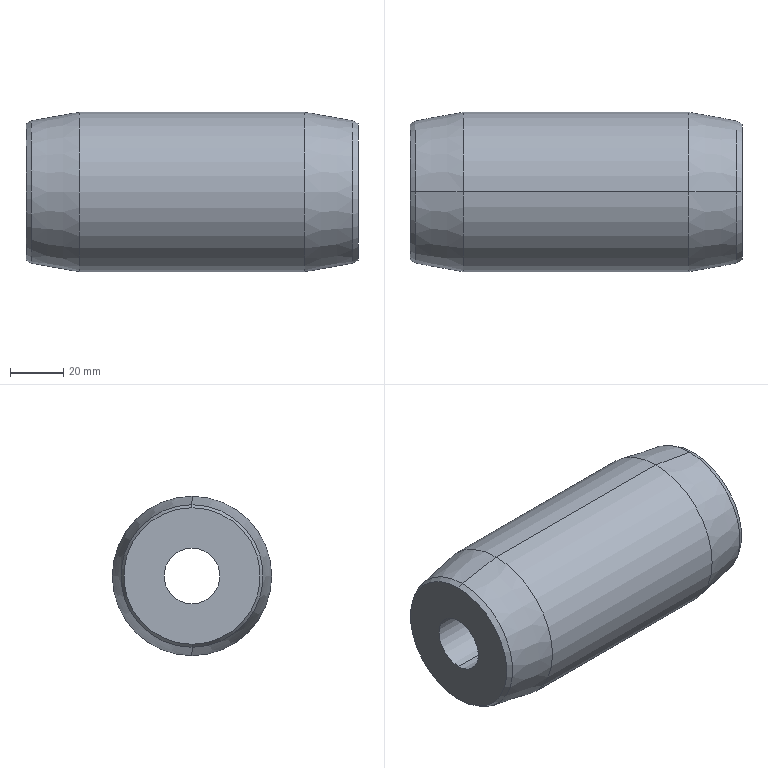Part | SolidWorks | features 3DProfileFeature 1, Chamfer 1, HoleWzd 1, ICE 1, Revolution 1 | 1 solid | 14 faces | box 125 x 60 x 60 mm | volume 297103 mm3 | cone 8 | cylinder 4 | plane 2 | commonest cylinder face diameters 21 x2 60 x2
STEP:
#1=CARTESIAN_POINT('',(125.,0.,-25.684));
#2=VERTEX_POINT('',#1);
#3=CARTESIAN_POINT('',(125.,0.,25.684));
#4=VERTEX_POINT('',#3);
#5=CARTESIAN_POINT('',(125.,0.,0.));
#6=DIRECTION('',(1.,0.,0.));
#7=DIRECTION('',(0.,0.,1.));
#8=AXIS2_PLACEMENT_3D('',#5,#6,#7);
#9=CIRCLE('',#8,25.684);
#10=EDGE_CURVE('',#2,#4,#9,.T.);
#11=ORIENTED_EDGE('',*,*,#10,.F.);
#12=CARTESIAN_POINT('',(123.03,0.,-26.821));
#13=VERTEX_POINT('',#12);
#14=CARTESIAN_POINT('',(123.03,0.,-26.821));
#15=DIRECTION('',(-0.866,0.,-0.5));
#16=VECTOR('',#15,1000.);
#17=LINE('',#14,#16);
#18=EDGE_CURVE('',#2,#13,#17,.T.);
#19=ORIENTED_EDGE('',*,*,#18,.T.);
#20=CARTESIAN_POINT('',(123.03,0.,26.821));
#21=VERTEX_POINT('',#20);
#22=CARTESIAN_POINT('',(123.03,0.,0.));
#23=DIRECTION('',(-1.,0.,0.));
#24=DIRECTION('',(0.,0.,-1.));
#25=AXIS2_PLACEMENT_3D('',#22,#23,#24);
#26=CIRCLE('',#25,26.821);
#27=EDGE_CURVE('',#21,#13,#26,.T.);
#28=ORIENTED_EDGE('',*,*,#27,.F.);
#29=CARTESIAN_POINT('',(123.03,0.,26.821));
#30=DIRECTION('',(-0.866,0.,0.5));
#31=VECTOR('',#30,1000.);
#32=LINE('',#29,#31);
#33=EDGE_CURVE('',#4,#21,#32,.T.);
#34=ORIENTED_EDGE('',*,*,#33,.F.);
#35=EDGE_LOOP('',(#11,#19,#28,#34));
#36=FACE_OUTER_BOUND('',#35,.T.);
#37=CARTESIAN_POINT('',(123.03,0.,0.));
#38=DIRECTION('',(-1.,0.,0.));
#39=DIRECTION('',(0.,0.,1.));
#40=AXIS2_PLACEMENT_3D('',#37,#38,#39);
#41=CONICAL_SURFACE('',#40,26.821,0.5236);
#42=ADVANCED_FACE('',(#36),#41,.T.);
#43=CARTESIAN_POINT('',(0.,0.,25.684));
#44=VERTEX_POINT('',#43);
#45=CARTESIAN_POINT('',(0.,0.,-25.684));
#46=VERTEX_POINT('',#45);
#47=CARTESIAN_POINT('',(0.,0.,0.));
#48=DIRECTION('',(-1.,0.,0.));
#49=DIRECTION('',(0.,0.,-1.));
#50=AXIS2_PLACEMENT_3D('',#47,#48,#49);
#51=CIRCLE('',#50,25.684);
#52=EDGE_CURVE('',#44,#46,#51,.T.);
#53=ORIENTED_EDGE('',*,*,#52,.F.);
#54=CARTESIAN_POINT('',(1.97,0.,26.821));
#55=VERTEX_POINT('',#54);
#56=CARTESIAN_POINT('',(0.,0.,25.684));
#57=DIRECTION('',(0.866,0.,0.5));
#58=VECTOR('',#57,1000.);
#59=LINE('',#56,#58);
#60=EDGE_CURVE('',#44,#55,#59,.T.);
#61=ORIENTED_EDGE('',*,*,#60,.T.);
#62=CARTESIAN_POINT('',(1.97,0.,-26.821));
#63=VERTEX_POINT('',#62);
#64=CARTESIAN_POINT('',(1.97,0.,0.));
#65=DIRECTION('',(1.,0.,0.));
#66=DIRECTION('',(0.,0.,1.));
#67=AXIS2_PLACEMENT_3D('',#64,#65,#66);
#68=CIRCLE('',#67,26.821);
#69=EDGE_CURVE('',#63,#55,#68,.T.);
#70=ORIENTED_EDGE('',*,*,#69,.F.);
#71=CARTESIAN_POINT('',(0.,0.,-25.684));
#72=DIRECTION('',(0.866,0.,-0.5));
#73=VECTOR('',#72,1000.);
#74=LINE('',#71,#73);
#75=EDGE_CURVE('',#46,#63,#74,.T.);
#76=ORIENTED_EDGE('',*,*,#75,.F.);
#77=EDGE_LOOP('',(#53,#61,#70,#76));
#78=FACE_OUTER_BOUND('',#77,.T.);
#79=CARTESIAN_POINT('',(0.,0.,0.));
#80=DIRECTION('',(1.,0.,0.));
#81=DIRECTION('',(0.,0.,-1.));
#82=AXIS2_PLACEMENT_3D('',#79,#80,#81);
#83=CONICAL_SURFACE('',#82,25.684,0.5236);
#84=ADVANCED_FACE('',(#78),#83,.T.);
#85=CARTESIAN_POINT('',(0.,0.,10.5));
#86=VERTEX_POINT('',#85);
#87=CARTESIAN_POINT('',(0.,0.,-10.5));
#88=VERTEX_POINT('',#87);
#89=CARTESIAN_POINT('',(0.,0.,0.));
#90=DIRECTION('',(1.,0.,0.));
#91=DIRECTION('',(0.,0.,-1.));
#92=AXIS2_PLACEMENT_3D('',#89,#90,#91);
#93=CIRCLE('',#92,10.5);
#94=EDGE_CURVE('',#86,#88,#93,.T.);
#95=ORIENTED_EDGE('',*,*,#94,.F.);
#96=CARTESIAN_POINT('',(125.,0.,10.5));
#97=VERTEX_POINT('',#96);
#98=CARTESIAN_POINT('',(0.,0.,10.5));
#99=DIRECTION('',(1.,0.,0.));
#100=VECTOR('',#99,1000.);
#101=LINE('',#98,#100);
#102=EDGE_CURVE('',#86,#97,#101,.T.);
#103=ORIENTED_EDGE('',*,*,#102,.T.);
#104=CARTESIAN_POINT('',(125.,0.,-10.5));
#105=VERTEX_POINT('',#104);
#106=CARTESIAN_POINT('',(125.,0.,0.));
#107=DIRECTION('',(1.,0.,0.));
#108=DIRECTION('',(0.,0.,-1.));
#109=AXIS2_PLACEMENT_3D('',#106,#107,#108);
#110=CIRCLE('',#109,10.5);
#111=EDGE_CURVE('',#97,#105,#110,.T.);
#112=ORIENTED_EDGE('',*,*,#111,.T.);
#113=CARTESIAN_POINT('',(0.,0.,-10.5));
#114=DIRECTION('',(1.,0.,0.));
#115=VECTOR('',#114,1000.);
#116=LINE('',#113,#115);
#117=EDGE_CURVE('',#88,#105,#116,.T.);
#118=ORIENTED_EDGE('',*,*,#117,.F.);
#119=EDGE_LOOP('',(#95,#103,#112,#118));
#120=FACE_OUTER_BOUND('',#119,.T.);
#121=CARTESIAN_POINT('',(0.,0.,0.));
#122=DIRECTION('',(1.,0.,0.));
#123=DIRECTION('',(0.,0.,-1.));
#124=AXIS2_PLACEMENT_3D('',#121,#122,#123);
#125=CYLINDRICAL_SURFACE('',#124,10.5);
#126=ADVANCED_FACE('',(#120),#125,.F.);
#127=ORIENTED_EDGE('',*,*,#69,.T.);
#128=CARTESIAN_POINT('',(20.,0.,30.));
#129=VERTEX_POINT('',#128);
#130=CARTESIAN_POINT('',(20.,0.,30.));
#131=DIRECTION('',(0.9848,0.,0.1736));
#132=VECTOR('',#131,1000.);
#133=LINE('',#130,#132);
#134=EDGE_CURVE('',#55,#129,#133,.T.);
#135=ORIENTED_EDGE('',*,*,#134,.T.);
#136=CARTESIAN_POINT('',(20.,0.,-30.));
#137=VERTEX_POINT('',#136);
#138=CARTESIAN_POINT('',(20.,0.,0.));
#139=DIRECTION('',(-1.,0.,0.));
#140=DIRECTION('',(0.,0.,1.));
#141=AXIS2_PLACEMENT_3D('',#138,#139,#140);
#142=CIRCLE('',#141,30.);
#143=EDGE_CURVE('',#129,#137,#142,.T.);
#144=ORIENTED_EDGE('',*,*,#143,.T.);
#145=CARTESIAN_POINT('',(20.,0.,-30.));
#146=DIRECTION('',(0.9848,0.,-0.1736));
#147=VECTOR('',#146,1000.);
#148=LINE('',#145,#147);
#149=EDGE_CURVE('',#63,#137,#148,.T.);
#150=ORIENTED_EDGE('',*,*,#149,.F.);
#151=EDGE_LOOP('',(#127,#135,#144,#150));
#152=FACE_OUTER_BOUND('',#151,.T.);
#153=CARTESIAN_POINT('',(20.,0.,0.));
#154=DIRECTION('',(1.,0.,0.));
#155=DIRECTION('',(0.,0.,-1.));
#156=AXIS2_PLACEMENT_3D('',#153,#154,#155);
#157=CONICAL_SURFACE('',#156,30.,0.1745);
#158=ADVANCED_FACE('',(#152),#157,.T.);
#159=CARTESIAN_POINT('',(105.,0.,30.));
#160=VERTEX_POINT('',#159);
#161=CARTESIAN_POINT('',(105.,0.,-30.));
#162=VERTEX_POINT('',#161);
#163=CARTESIAN_POINT('',(105.,0.,0.));
#164=DIRECTION('',(-1.,0.,0.));
#165=DIRECTION('',(0.,0.,1.));
#166=AXIS2_PLACEMENT_3D('',#163,#164,#165);
#167=CIRCLE('',#166,30.);
#168=EDGE_CURVE('',#160,#162,#167,.T.);
#169=ORIENTED_EDGE('',*,*,#168,.T.);
#170=CARTESIAN_POINT('',(0.,0.,-30.));
#171=DIRECTION('',(-1.,0.,0.));
#172=VECTOR('',#171,1000.);
#173=LINE('',#170,#172);
#174=EDGE_CURVE('',#162,#137,#173,.T.);
#175=ORIENTED_EDGE('',*,*,#174,.T.);
#176=ORIENTED_EDGE('',*,*,#143,.F.);
#177=CARTESIAN_POINT('',(0.,0.,30.));
#178=DIRECTION('',(-1.,0.,0.));
#179=VECTOR('',#178,1000.);
#180=LINE('',#177,#179);
#181=EDGE_CURVE('',#160,#129,#180,.T.);
#182=ORIENTED_EDGE('',*,*,#181,.F.);
#183=EDGE_LOOP('',(#169,#175,#176,#182));
#184=FACE_OUTER_BOUND('',#183,.T.);
#185=CARTESIAN_POINT('',(0.,0.,0.));
#186=DIRECTION('',(-1.,0.,0.));
#187=DIRECTION('',(0.,0.,1.));
#188=AXIS2_PLACEMENT_3D('',#185,#186,#187);
#189=CYLINDRICAL_SURFACE('',#188,30.);
#190=ADVANCED_FACE('',(#184),#189,.T.);
#191=ORIENTED_EDGE('',*,*,#27,.T.);
#192=CARTESIAN_POINT('',(125.,0.,-26.473));
#193=DIRECTION('',(-0.9848,0.,-0.1736));
#194=VECTOR('',#193,1000.);
#195=LINE('',#192,#194);
#196=EDGE_CURVE('',#13,#162,#195,.T.);
#197=ORIENTED_EDGE('',*,*,#196,.T.);
#198=ORIENTED_EDGE('',*,*,#168,.F.);
#199=CARTESIAN_POINT('',(125.,0.,26.473));
#200=DIRECTION('',(-0.9848,0.,0.1736));
#201=VECTOR('',#200,1000.);
#202=LINE('',#199,#201);
#203=EDGE_CURVE('',#21,#160,#202,.T.);
#204=ORIENTED_EDGE('',*,*,#203,.F.);
#205=EDGE_LOOP('',(#191,#197,#198,#204));
#206=FACE_OUTER_BOUND('',#205,.T.);
#207=CARTESIAN_POINT('',(125.,0.,0.));
#208=DIRECTION('',(-1.,0.,0.));
#209=DIRECTION('',(0.,0.,1.));
#210=AXIS2_PLACEMENT_3D('',#207,#208,#209);
#211=CONICAL_SURFACE('',#210,26.473,0.1745);
#212=ADVANCED_FACE('',(#206),#211,.T.);
#213=CARTESIAN_POINT('',(125.,0.,0.));
#214=DIRECTION('',(1.,0.,0.));
#215=DIRECTION('',(0.,0.,1.));
#216=AXIS2_PLACEMENT_3D('',#213,#214,#215);
#217=CIRCLE('',#216,25.684);
#218=EDGE_CURVE('',#4,#2,#217,.T.);
#219=ORIENTED_EDGE('',*,*,#218,.T.);
#220=ORIENTED_EDGE('',*,*,#10,.T.);
#221=EDGE_LOOP('',(#219,#220));
#222=FACE_OUTER_BOUND('',#221,.T.);
#223=CARTESIAN_POINT('',(125.,0.,0.));
#224=DIRECTION('',(1.,0.,0.));
#225=DIRECTION('',(0.,0.,-1.));
#226=AXIS2_PLACEMENT_3D('',#223,#224,#225);
#227=CIRCLE('',#226,10.5);
#228=EDGE_CURVE('',#105,#97,#227,.T.);
#229=ORIENTED_EDGE('',*,*,#228,.F.);
#230=ORIENTED_EDGE('',*,*,#111,.F.);
#231=EDGE_LOOP('',(#229,#230));
#232=FACE_BOUND('',#231,.T.);
#233=CARTESIAN_POINT('',(125.,0.,0.));
#234=DIRECTION('',(-1.,0.,0.));
#235=DIRECTION('',(0.,0.,1.));
#236=AXIS2_PLACEMENT_3D('',#233,#234,#235);
#237=PLANE('',#236);
#238=ADVANCED_FACE('',(#222,#232),#237,.F.);
#239=ORIENTED_EDGE('',*,*,#196,.F.);
#240=CARTESIAN_POINT('',(123.03,0.,0.));
#241=DIRECTION('',(-1.,0.,0.));
#242=DIRECTION('',(0.,0.,-1.));
#243=AXIS2_PLACEMENT_3D('',#240,#241,#242);
#244=CIRCLE('',#243,26.821);
#245=EDGE_CURVE('',#13,#21,#244,.T.);
#246=ORIENTED_EDGE('',*,*,#245,.T.);
#247=ORIENTED_EDGE('',*,*,#203,.T.);
#248=CARTESIAN_POINT('',(105.,0.,0.));
#249=DIRECTION('',(-1.,0.,0.));
#250=DIRECTION('',(0.,0.,1.));
#251=AXIS2_PLACEMENT_3D('',#248,#249,#250);
#252=CIRCLE('',#251,30.);
#253=EDGE_CURVE('',#162,#160,#252,.T.);
#254=ORIENTED_EDGE('',*,*,#253,.F.);
#255=EDGE_LOOP('',(#239,#246,#247,#254));
#256=FACE_OUTER_BOUND('',#255,.T.);
#257=CARTESIAN_POINT('',(125.,0.,0.));
#258=DIRECTION('',(-1.,0.,0.));
#259=DIRECTION('',(0.,0.,1.));
#260=AXIS2_PLACEMENT_3D('',#257,#258,#259);
#261=CONICAL_SURFACE('',#260,26.473,0.1745);
#262=ADVANCED_FACE('',(#256),#261,.T.);
#263=ORIENTED_EDGE('',*,*,#174,.F.);
#264=ORIENTED_EDGE('',*,*,#253,.T.);
#265=ORIENTED_EDGE('',*,*,#181,.T.);
#266=CARTESIAN_POINT('',(20.,0.,0.));
#267=DIRECTION('',(-1.,0.,0.));
#268=DIRECTION('',(0.,0.,1.));
#269=AXIS2_PLACEMENT_3D('',#266,#267,#268);
#270=CIRCLE('',#269,30.);
#271=EDGE_CURVE('',#137,#129,#270,.T.);
#272=ORIENTED_EDGE('',*,*,#271,.F.);
#273=EDGE_LOOP('',(#263,#264,#265,#272));
#274=FACE_OUTER_BOUND('',#273,.T.);
#275=CARTESIAN_POINT('',(0.,0.,0.));
#276=DIRECTION('',(-1.,0.,0.));
#277=DIRECTION('',(0.,0.,1.));
#278=AXIS2_PLACEMENT_3D('',#275,#276,#277);
#279=CYLINDRICAL_SURFACE('',#278,30.);
#280=ADVANCED_FACE('',(#274),#279,.T.);
#281=ORIENTED_EDGE('',*,*,#134,.F.);
#282=CARTESIAN_POINT('',(1.97,0.,0.));
#283=DIRECTION('',(1.,0.,0.));
#284=DIRECTION('',(0.,0.,1.));
#285=AXIS2_PLACEMENT_3D('',#282,#283,#284);
#286=CIRCLE('',#285,26.821);
#287=EDGE_CURVE('',#55,#63,#286,.T.);
#288=ORIENTED_EDGE('',*,*,#287,.T.);
#289=ORIENTED_EDGE('',*,*,#149,.T.);
#290=ORIENTED_EDGE('',*,*,#271,.T.);
#291=EDGE_LOOP('',(#281,#288,#289,#290));
#292=FACE_OUTER_BOUND('',#291,.T.);
#293=CARTESIAN_POINT('',(20.,0.,0.));
#294=DIRECTION('',(1.,0.,0.));
#295=DIRECTION('',(0.,0.,-1.));
#296=AXIS2_PLACEMENT_3D('',#293,#294,#295);
#297=CONICAL_SURFACE('',#296,30.,0.1745);
#298=ADVANCED_FACE('',(#292),#297,.T.);
#299=CARTESIAN_POINT('',(0.,0.,0.));
#300=DIRECTION('',(-1.,0.,0.));
#301=DIRECTION('',(0.,0.,-1.));
#302=AXIS2_PLACEMENT_3D('',#299,#300,#301);
#303=CIRCLE('',#302,25.684);
#304=EDGE_CURVE('',#46,#44,#303,.T.);
#305=ORIENTED_EDGE('',*,*,#304,.T.);
#306=ORIENTED_EDGE('',*,*,#52,.T.);
#307=EDGE_LOOP('',(#305,#306));
#308=FACE_OUTER_BOUND('',#307,.T.);
#309=CARTESIAN_POINT('',(0.,0.,0.));
#310=DIRECTION('',(1.,0.,0.));
#311=DIRECTION('',(0.,0.,-1.));
#312=AXIS2_PLACEMENT_3D('',#309,#310,#311);
#313=CIRCLE('',#312,10.5);
#314=EDGE_CURVE('',#88,#86,#313,.T.);
#315=ORIENTED_EDGE('',*,*,#314,.T.);
#316=ORIENTED_EDGE('',*,*,#94,.T.);
#317=EDGE_LOOP('',(#315,#316));
#318=FACE_BOUND('',#317,.T.);
#319=CARTESIAN_POINT('',(0.,0.,0.));
#320=DIRECTION('',(1.,0.,0.));
#321=DIRECTION('',(0.,0.,-1.));
#322=AXIS2_PLACEMENT_3D('',#319,#320,#321);
#323=PLANE('',#322);
#324=ADVANCED_FACE('',(#308,#318),#323,.F.);
#325=ORIENTED_EDGE('',*,*,#102,.F.);
#326=ORIENTED_EDGE('',*,*,#314,.F.);
#327=ORIENTED_EDGE('',*,*,#117,.T.);
#328=ORIENTED_EDGE('',*,*,#228,.T.);
#329=EDGE_LOOP('',(#325,#326,#327,#328));
#330=FACE_OUTER_BOUND('',#329,.T.);
#331=CARTESIAN_POINT('',(0.,0.,0.));
#332=DIRECTION('',(1.,0.,0.));
#333=DIRECTION('',(0.,0.,-1.));
#334=AXIS2_PLACEMENT_3D('',#331,#332,#333);
#335=CYLINDRICAL_SURFACE('',#334,10.5);
#336=ADVANCED_FACE('',(#330),#335,.F.);
#337=ORIENTED_EDGE('',*,*,#60,.F.);
#338=ORIENTED_EDGE('',*,*,#304,.F.);
#339=ORIENTED_EDGE('',*,*,#75,.T.);
#340=ORIENTED_EDGE('',*,*,#287,.F.);
#341=EDGE_LOOP('',(#337,#338,#339,#340));
#342=FACE_OUTER_BOUND('',#341,.T.);
#343=CARTESIAN_POINT('',(0.,0.,0.));
#344=DIRECTION('',(1.,0.,0.));
#345=DIRECTION('',(0.,0.,-1.));
#346=AXIS2_PLACEMENT_3D('',#343,#344,#345);
#347=CONICAL_SURFACE('',#346,25.684,0.5236);
#348=ADVANCED_FACE('',(#342),#347,.T.);
#349=ORIENTED_EDGE('',*,*,#18,.F.);
#350=ORIENTED_EDGE('',*,*,#218,.F.);
#351=ORIENTED_EDGE('',*,*,#33,.T.);
#352=ORIENTED_EDGE('',*,*,#245,.F.);
#353=EDGE_LOOP('',(#349,#350,#351,#352));
#354=FACE_OUTER_BOUND('',#353,.T.);
#355=CARTESIAN_POINT('',(123.03,0.,0.));
#356=DIRECTION('',(-1.,0.,0.));
#357=DIRECTION('',(0.,0.,1.));
#358=AXIS2_PLACEMENT_3D('',#355,#356,#357);
#359=CONICAL_SURFACE('',#358,26.821,0.5236);
#360=ADVANCED_FACE('',(#354),#359,.T.);
#361=CLOSED_SHELL('',(#42,#84,#126,#158,#190,#212,#238,#262,#280,#298,#324,#336,#348,#360));
#362=MANIFOLD_SOLID_BREP('',#361);
#363=CARTESIAN_POINT('',(0.,0.,0.));
#364=DIRECTION('',(0.,0.,1.));
#365=DIRECTION('',(1.,0.,0.));
#366=AXIS2_PLACEMENT_3D('',#363,#364,#365);
#367=(LENGTH_UNIT()NAMED_UNIT(*)SI_UNIT(.MILLI.,.METRE.));
#368=UNCERTAINTY_MEASURE_WITH_UNIT(LENGTH_MEASURE(0.00001),#367,'','');
#369=(NAMED_UNIT(*)PLANE_ANGLE_UNIT()SI_UNIT($,.RADIAN.));
#370=(NAMED_UNIT(*)SI_UNIT($,.STERADIAN.)SOLID_ANGLE_UNIT());
#371=(GEOMETRIC_REPRESENTATION_CONTEXT(3)GLOBAL_UNCERTAINTY_ASSIGNED_CONTEXT((#368))GLOBAL_UNIT_ASSIGNED_CONTEXT((#367,#369,#370))REPRESENTATION_CONTEXT('',''));
#372=ADVANCED_BREP_SHAPE_REPRESENTATION('',(#362,#366),#371);